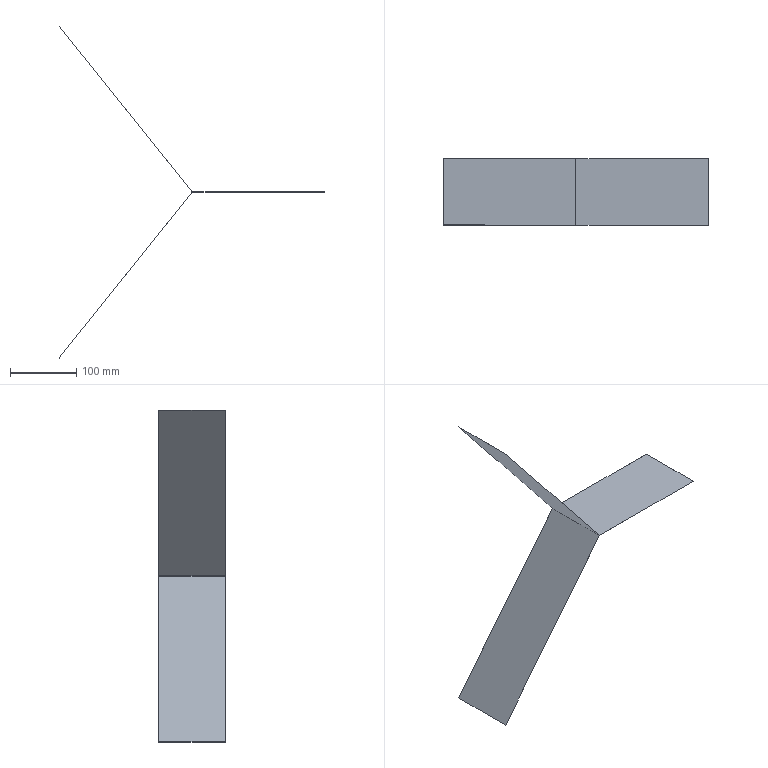Part | STEP file | A14-Product-1 | 1 solid | 11 faces | box 399.758 x 100 x 500.012 mm | volume 1680 mm3 | plane 11
STEP:
#1=CARTESIAN_POINT('',(0.,0.,0.));
#2=DIRECTION('',(0.,0.,1.));
#3=DIRECTION('',(1.,0.,0.));
#4=AXIS2_PLACEMENT_3D('',#1,#2,#3);
#5=CARTESIAN_POINT('',(199.755,-50.,0.01));
#6=VERTEX_POINT('',#5);
#7=CARTESIAN_POINT('',(399.75,-50.,0.01));
#8=VERTEX_POINT('',#7);
#9=CARTESIAN_POINT('',(199.75,-50.,0.01));
#10=DIRECTION('',(1.,0.,0.));
#11=VECTOR('',#10,1.);
#12=LINE('',#9,#11);
#13=CARTESIAN_POINT('',(0.,-50.,0.));
#14=DIRECTION('',(0.,-1.,0.));
#15=DIRECTION('',(-1.,0.,0.));
#16=AXIS2_PLACEMENT_3D('',#13,#14,#15);
#17=PLANE('',#16);
#18=CARTESIAN_POINT('',(-199.75,-0.01));
#19=DIRECTION('',(-1.,0.));
#20=VECTOR('',#19,1.);
#21=LINE('',#18,#20);
#22=(GEOMETRIC_REPRESENTATION_CONTEXT(2)PARAMETRIC_REPRESENTATION_CONTEXT()REPRESENTATION_CONTEXT('',''));
#23=DEFINITIONAL_REPRESENTATION('',(#21),#22);
#24=PCURVE('',#17,#23);
#25=CARTESIAN_POINT('',(199.75,50.,0.01));
#26=DIRECTION('',(0.,0.,-1.));
#27=DIRECTION('',(-1.,0.,0.));
#28=AXIS2_PLACEMENT_3D('',#25,#26,#27);
#29=PLANE('',#28);
#30=CARTESIAN_POINT('',(0.,-100.));
#31=DIRECTION('',(-1.,0.));
#32=VECTOR('',#31,1.);
#33=LINE('',#30,#32);
#34=(GEOMETRIC_REPRESENTATION_CONTEXT(2)PARAMETRIC_REPRESENTATION_CONTEXT()REPRESENTATION_CONTEXT('',''));
#35=DEFINITIONAL_REPRESENTATION('',(#33),#34);
#36=PCURVE('',#29,#35);
#37=SURFACE_CURVE('',#12,(#24,#36),.PCURVE_S1.);
#38=EDGE_CURVE('',#6,#8,#37,.T.);
#39=ORIENTED_EDGE('',*,*,#38,.F.);
#40=CARTESIAN_POINT('',(0.007812,-50.,250.006));
#41=VERTEX_POINT('',#40);
#42=CARTESIAN_POINT('',(199.758,-50.,0.006242));
#43=DIRECTION('',(-0.6242,0.,0.7812));
#44=VECTOR('',#43,1.);
#45=LINE('',#42,#44);
#46=CARTESIAN_POINT('',(-199.758,-0.006242));
#47=DIRECTION('',(0.6242,-0.7812));
#48=VECTOR('',#47,1.);
#49=LINE('',#46,#48);
#50=(GEOMETRIC_REPRESENTATION_CONTEXT(2)PARAMETRIC_REPRESENTATION_CONTEXT()REPRESENTATION_CONTEXT('',''));
#51=DEFINITIONAL_REPRESENTATION('',(#49),#50);
#52=PCURVE('',#17,#51);
#53=CARTESIAN_POINT('',(199.758,50.,0.006242));
#54=DIRECTION('',(0.7812,0.,0.6242));
#55=DIRECTION('',(0.6242,0.,-0.7812));
#56=AXIS2_PLACEMENT_3D('',#53,#54,#55);
#57=PLANE('',#56);
#58=CARTESIAN_POINT('',(0.,-100.));
#59=DIRECTION('',(-1.,0.));
#60=VECTOR('',#59,1.);
#61=LINE('',#58,#60);
#62=(GEOMETRIC_REPRESENTATION_CONTEXT(2)PARAMETRIC_REPRESENTATION_CONTEXT()REPRESENTATION_CONTEXT('',''));
#63=DEFINITIONAL_REPRESENTATION('',(#61),#62);
#64=PCURVE('',#57,#63);
#65=SURFACE_CURVE('',#45,(#52,#64),.PCURVE_S1.);
#66=EDGE_CURVE('',#6,#41,#65,.T.);
#67=ORIENTED_EDGE('',*,*,#66,.T.);
#68=CARTESIAN_POINT('',(-0.007813,-50.,249.994));
#69=VERTEX_POINT('',#68);
#70=CARTESIAN_POINT('',(0.007812,-50.,250.006));
#71=DIRECTION('',(-0.7812,0.,-0.6242));
#72=VECTOR('',#71,1.);
#73=LINE('',#70,#72);
#74=CARTESIAN_POINT('',(-0.007812,-250.006));
#75=DIRECTION('',(0.7812,0.6242));
#76=VECTOR('',#75,1.);
#77=LINE('',#74,#76);
#78=(GEOMETRIC_REPRESENTATION_CONTEXT(2)PARAMETRIC_REPRESENTATION_CONTEXT()REPRESENTATION_CONTEXT('',''));
#79=DEFINITIONAL_REPRESENTATION('',(#77),#78);
#80=PCURVE('',#17,#79);
#81=CARTESIAN_POINT('',(0.007812,50.,250.006));
#82=DIRECTION('',(-0.6242,0.,0.7812));
#83=DIRECTION('',(0.7812,0.,0.6242));
#84=AXIS2_PLACEMENT_3D('',#81,#82,#83);
#85=PLANE('',#84);
#86=CARTESIAN_POINT('',(0.,-100.));
#87=DIRECTION('',(-1.,0.));
#88=VECTOR('',#87,1.);
#89=LINE('',#86,#88);
#90=(GEOMETRIC_REPRESENTATION_CONTEXT(2)PARAMETRIC_REPRESENTATION_CONTEXT()REPRESENTATION_CONTEXT('',''));
#91=DEFINITIONAL_REPRESENTATION('',(#89),#90);
#92=PCURVE('',#85,#91);
#93=SURFACE_CURVE('',#73,(#80,#92),.PCURVE_S1.);
#94=EDGE_CURVE('',#41,#69,#93,.T.);
#95=ORIENTED_EDGE('',*,*,#94,.T.);
#96=CARTESIAN_POINT('',(199.737,-50.,0.));
#97=VERTEX_POINT('',#96);
#98=CARTESIAN_POINT('',(199.742,-50.,-0.006242));
#99=DIRECTION('',(-0.6242,0.,0.7812));
#100=VECTOR('',#99,1.);
#101=LINE('',#98,#100);
#102=CARTESIAN_POINT('',(-199.742,0.006242));
#103=DIRECTION('',(0.6242,-0.7812));
#104=VECTOR('',#103,1.);
#105=LINE('',#102,#104);
#106=(GEOMETRIC_REPRESENTATION_CONTEXT(2)PARAMETRIC_REPRESENTATION_CONTEXT()REPRESENTATION_CONTEXT('',''));
#107=DEFINITIONAL_REPRESENTATION('',(#105),#106);
#108=PCURVE('',#17,#107);
#109=CARTESIAN_POINT('',(199.742,50.,-0.006242));
#110=DIRECTION('',(0.7812,0.,0.6242));
#111=DIRECTION('',(0.6242,0.,-0.7812));
#112=AXIS2_PLACEMENT_3D('',#109,#110,#111);
#113=PLANE('',#112);
#114=CARTESIAN_POINT('',(0.,-100.));
#115=DIRECTION('',(-1.,0.));
#116=VECTOR('',#115,1.);
#117=LINE('',#114,#116);
#118=(GEOMETRIC_REPRESENTATION_CONTEXT(2)PARAMETRIC_REPRESENTATION_CONTEXT()REPRESENTATION_CONTEXT('',''));
#119=DEFINITIONAL_REPRESENTATION('',(#117),#118);
#120=PCURVE('',#113,#119);
#121=SURFACE_CURVE('',#101,(#108,#120),.PCURVE_S1.);
#122=EDGE_CURVE('',#97,#69,#121,.T.);
#123=ORIENTED_EDGE('',*,*,#122,.F.);
#124=CARTESIAN_POINT('',(-0.007812,-50.,-249.994));
#125=VERTEX_POINT('',#124);
#126=CARTESIAN_POINT('',(-0.007812,-50.,-249.994));
#127=DIRECTION('',(0.6242,0.,0.7812));
#128=VECTOR('',#127,1.);
#129=LINE('',#126,#128);
#130=CARTESIAN_POINT('',(0.007812,249.994));
#131=DIRECTION('',(-0.6242,-0.7812));
#132=VECTOR('',#131,1.);
#133=LINE('',#130,#132);
#134=(GEOMETRIC_REPRESENTATION_CONTEXT(2)PARAMETRIC_REPRESENTATION_CONTEXT()REPRESENTATION_CONTEXT('',''));
#135=DEFINITIONAL_REPRESENTATION('',(#133),#134);
#136=PCURVE('',#17,#135);
#137=CARTESIAN_POINT('',(-0.007812,50.,-249.994));
#138=DIRECTION('',(0.7812,0.,-0.6242));
#139=DIRECTION('',(-0.6242,0.,-0.7812));
#140=AXIS2_PLACEMENT_3D('',#137,#138,#139);
#141=PLANE('',#140);
#142=CARTESIAN_POINT('',(0.,-100.));
#143=DIRECTION('',(-1.,0.));
#144=VECTOR('',#143,1.);
#145=LINE('',#142,#144);
#146=(GEOMETRIC_REPRESENTATION_CONTEXT(2)PARAMETRIC_REPRESENTATION_CONTEXT()REPRESENTATION_CONTEXT('',''));
#147=DEFINITIONAL_REPRESENTATION('',(#145),#146);
#148=PCURVE('',#141,#147);
#149=SURFACE_CURVE('',#129,(#136,#148),.PCURVE_S1.);
#150=EDGE_CURVE('',#125,#97,#149,.T.);
#151=ORIENTED_EDGE('',*,*,#150,.F.);
#152=CARTESIAN_POINT('',(0.007813,-50.,-250.006));
#153=VERTEX_POINT('',#152);
#154=CARTESIAN_POINT('',(-0.007812,-50.,-249.994));
#155=DIRECTION('',(0.7812,0.,-0.6242));
#156=VECTOR('',#155,1.);
#157=LINE('',#154,#156);
#158=CARTESIAN_POINT('',(0.007812,249.994));
#159=DIRECTION('',(-0.7812,0.6242));
#160=VECTOR('',#159,1.);
#161=LINE('',#158,#160);
#162=(GEOMETRIC_REPRESENTATION_CONTEXT(2)PARAMETRIC_REPRESENTATION_CONTEXT()REPRESENTATION_CONTEXT('',''));
#163=DEFINITIONAL_REPRESENTATION('',(#161),#162);
#164=PCURVE('',#17,#163);
#165=CARTESIAN_POINT('',(-0.007812,50.,-249.994));
#166=DIRECTION('',(-0.6242,0.,-0.7812));
#167=DIRECTION('',(-0.7812,0.,0.6242));
#168=AXIS2_PLACEMENT_3D('',#165,#166,#167);
#169=PLANE('',#168);
#170=CARTESIAN_POINT('',(0.,-100.));
#171=DIRECTION('',(-1.,0.));
#172=VECTOR('',#171,1.);
#173=LINE('',#170,#172);
#174=(GEOMETRIC_REPRESENTATION_CONTEXT(2)PARAMETRIC_REPRESENTATION_CONTEXT()REPRESENTATION_CONTEXT('',''));
#175=DEFINITIONAL_REPRESENTATION('',(#173),#174);
#176=PCURVE('',#169,#175);
#177=SURFACE_CURVE('',#157,(#164,#176),.PCURVE_S1.);
#178=EDGE_CURVE('',#125,#153,#177,.T.);
#179=ORIENTED_EDGE('',*,*,#178,.T.);
#180=CARTESIAN_POINT('',(199.755,-50.,-0.01));
#181=VERTEX_POINT('',#180);
#182=CARTESIAN_POINT('',(0.007813,-50.,-250.006));
#183=DIRECTION('',(0.6242,0.,0.7812));
#184=VECTOR('',#183,1.);
#185=LINE('',#182,#184);
#186=CARTESIAN_POINT('',(-0.007813,250.006));
#187=DIRECTION('',(-0.6242,-0.7812));
#188=VECTOR('',#187,1.);
#189=LINE('',#186,#188);
#190=(GEOMETRIC_REPRESENTATION_CONTEXT(2)PARAMETRIC_REPRESENTATION_CONTEXT()REPRESENTATION_CONTEXT('',''));
#191=DEFINITIONAL_REPRESENTATION('',(#189),#190);
#192=PCURVE('',#17,#191);
#193=CARTESIAN_POINT('',(0.007813,50.,-250.006));
#194=DIRECTION('',(0.7812,0.,-0.6242));
#195=DIRECTION('',(-0.6242,0.,-0.7812));
#196=AXIS2_PLACEMENT_3D('',#193,#194,#195);
#197=PLANE('',#196);
#198=CARTESIAN_POINT('',(0.,-100.));
#199=DIRECTION('',(-1.,0.));
#200=VECTOR('',#199,1.);
#201=LINE('',#198,#200);
#202=(GEOMETRIC_REPRESENTATION_CONTEXT(2)PARAMETRIC_REPRESENTATION_CONTEXT()REPRESENTATION_CONTEXT('',''));
#203=DEFINITIONAL_REPRESENTATION('',(#201),#202);
#204=PCURVE('',#197,#203);
#205=SURFACE_CURVE('',#185,(#192,#204),.PCURVE_S1.);
#206=EDGE_CURVE('',#153,#181,#205,.T.);
#207=ORIENTED_EDGE('',*,*,#206,.T.);
#208=CARTESIAN_POINT('',(399.75,-50.,-0.01));
#209=VERTEX_POINT('',#208);
#210=CARTESIAN_POINT('',(199.75,-50.,-0.01));
#211=DIRECTION('',(1.,0.,0.));
#212=VECTOR('',#211,1.);
#213=LINE('',#210,#212);
#214=CARTESIAN_POINT('',(-199.75,0.01));
#215=DIRECTION('',(-1.,0.));
#216=VECTOR('',#215,1.);
#217=LINE('',#214,#216);
#218=(GEOMETRIC_REPRESENTATION_CONTEXT(2)PARAMETRIC_REPRESENTATION_CONTEXT()REPRESENTATION_CONTEXT('',''));
#219=DEFINITIONAL_REPRESENTATION('',(#217),#218);
#220=PCURVE('',#17,#219);
#221=CARTESIAN_POINT('',(199.75,50.,-0.01));
#222=DIRECTION('',(0.,0.,-1.));
#223=DIRECTION('',(-1.,0.,0.));
#224=AXIS2_PLACEMENT_3D('',#221,#222,#223);
#225=PLANE('',#224);
#226=CARTESIAN_POINT('',(0.,-100.));
#227=DIRECTION('',(-1.,0.));
#228=VECTOR('',#227,1.);
#229=LINE('',#226,#228);
#230=(GEOMETRIC_REPRESENTATION_CONTEXT(2)PARAMETRIC_REPRESENTATION_CONTEXT()REPRESENTATION_CONTEXT('',''));
#231=DEFINITIONAL_REPRESENTATION('',(#229),#230);
#232=PCURVE('',#225,#231);
#233=SURFACE_CURVE('',#213,(#220,#232),.PCURVE_S1.);
#234=EDGE_CURVE('',#181,#209,#233,.T.);
#235=ORIENTED_EDGE('',*,*,#234,.T.);
#236=CARTESIAN_POINT('',(399.75,-50.,-0.01));
#237=DIRECTION('',(0.,0.,1.));
#238=VECTOR('',#237,1.);
#239=LINE('',#236,#238);
#240=CARTESIAN_POINT('',(-399.75,0.01));
#241=DIRECTION('',(0.,-1.));
#242=VECTOR('',#241,1.);
#243=LINE('',#240,#242);
#244=(GEOMETRIC_REPRESENTATION_CONTEXT(2)PARAMETRIC_REPRESENTATION_CONTEXT()REPRESENTATION_CONTEXT('',''));
#245=DEFINITIONAL_REPRESENTATION('',(#243),#244);
#246=PCURVE('',#17,#245);
#247=CARTESIAN_POINT('',(399.75,50.,-0.01));
#248=DIRECTION('',(1.,0.,0.));
#249=DIRECTION('',(0.,0.,-1.));
#250=AXIS2_PLACEMENT_3D('',#247,#248,#249);
#251=PLANE('',#250);
#252=CARTESIAN_POINT('',(0.,-100.));
#253=DIRECTION('',(-1.,0.));
#254=VECTOR('',#253,1.);
#255=LINE('',#252,#254);
#256=(GEOMETRIC_REPRESENTATION_CONTEXT(2)PARAMETRIC_REPRESENTATION_CONTEXT()REPRESENTATION_CONTEXT('',''));
#257=DEFINITIONAL_REPRESENTATION('',(#255),#256);
#258=PCURVE('',#251,#257);
#259=SURFACE_CURVE('',#239,(#246,#258),.PCURVE_S1.);
#260=EDGE_CURVE('',#209,#8,#259,.T.);
#261=ORIENTED_EDGE('',*,*,#260,.T.);
#262=EDGE_LOOP('',(#39,#67,#95,#123,#151,#179,#207,#235,#261));
#263=FACE_BOUND('',#262,.T.);
#264=ADVANCED_FACE('',(#263),#17,.T.);
#265=CARTESIAN_POINT('',(199.755,50.,-0.01));
#266=VERTEX_POINT('',#265);
#267=CARTESIAN_POINT('',(199.755,50.,-0.01));
#268=DIRECTION('',(0.,1.,0.));
#269=VECTOR('',#268,1.);
#270=LINE('',#267,#269);
#271=CARTESIAN_POINT('',(-319.995,0.));
#272=DIRECTION('',(0.,1.));
#273=VECTOR('',#272,1.);
#274=LINE('',#271,#273);
#275=(GEOMETRIC_REPRESENTATION_CONTEXT(2)PARAMETRIC_REPRESENTATION_CONTEXT()REPRESENTATION_CONTEXT('',''));
#276=DEFINITIONAL_REPRESENTATION('',(#274),#275);
#277=PCURVE('',#197,#276);
#278=CARTESIAN_POINT('',(-0.00481,0.));
#279=DIRECTION('',(0.,1.));
#280=VECTOR('',#279,1.);
#281=LINE('',#278,#280);
#282=(GEOMETRIC_REPRESENTATION_CONTEXT(2)PARAMETRIC_REPRESENTATION_CONTEXT()REPRESENTATION_CONTEXT('',''));
#283=DEFINITIONAL_REPRESENTATION('',(#281),#282);
#284=PCURVE('',#225,#283);
#285=SURFACE_CURVE('',#270,(#277,#284),.PCURVE_S1.);
#286=EDGE_CURVE('',#181,#266,#285,.T.);
#287=ORIENTED_EDGE('',*,*,#286,.F.);
#288=ORIENTED_EDGE('',*,*,#206,.F.);
#289=CARTESIAN_POINT('',(0.007813,50.,-250.006));
#290=VERTEX_POINT('',#289);
#291=CARTESIAN_POINT('',(0.007813,50.,-250.006));
#292=DIRECTION('',(0.,-1.,0.));
#293=VECTOR('',#292,1.);
#294=LINE('',#291,#293);
#295=CARTESIAN_POINT('',(0.,0.));
#296=DIRECTION('',(0.,-1.));
#297=VECTOR('',#296,1.);
#298=LINE('',#295,#297);
#299=(GEOMETRIC_REPRESENTATION_CONTEXT(2)PARAMETRIC_REPRESENTATION_CONTEXT()REPRESENTATION_CONTEXT('',''));
#300=DEFINITIONAL_REPRESENTATION('',(#298),#299);
#301=PCURVE('',#197,#300);
#302=CARTESIAN_POINT('',(-0.02,0.));
#303=DIRECTION('',(0.,-1.));
#304=VECTOR('',#303,1.);
#305=LINE('',#302,#304);
#306=(GEOMETRIC_REPRESENTATION_CONTEXT(2)PARAMETRIC_REPRESENTATION_CONTEXT()REPRESENTATION_CONTEXT('',''));
#307=DEFINITIONAL_REPRESENTATION('',(#305),#306);
#308=PCURVE('',#169,#307);
#309=SURFACE_CURVE('',#294,(#301,#308),.PCURVE_S1.);
#310=EDGE_CURVE('',#290,#153,#309,.T.);
#311=ORIENTED_EDGE('',*,*,#310,.F.);
#312=CARTESIAN_POINT('',(0.007813,50.,-250.006));
#313=DIRECTION('',(0.6242,0.,0.7812));
#314=VECTOR('',#313,1.);
#315=LINE('',#312,#314);
#316=CARTESIAN_POINT('',(0.,0.));
#317=DIRECTION('',(-1.,0.));
#318=VECTOR('',#317,1.);
#319=LINE('',#316,#318);
#320=(GEOMETRIC_REPRESENTATION_CONTEXT(2)PARAMETRIC_REPRESENTATION_CONTEXT()REPRESENTATION_CONTEXT('',''));
#321=DEFINITIONAL_REPRESENTATION('',(#319),#320);
#322=PCURVE('',#197,#321);
#323=CARTESIAN_POINT('',(0.,50.,0.));
#324=DIRECTION('',(0.,-1.,0.));
#325=DIRECTION('',(-1.,0.,0.));
#326=AXIS2_PLACEMENT_3D('',#323,#324,#325);
#327=PLANE('',#326);
#328=CARTESIAN_POINT('',(-0.007813,250.006));
#329=DIRECTION('',(-0.6242,-0.7812));
#330=VECTOR('',#329,1.);
#331=LINE('',#328,#330);
#332=(GEOMETRIC_REPRESENTATION_CONTEXT(2)PARAMETRIC_REPRESENTATION_CONTEXT()REPRESENTATION_CONTEXT('',''));
#333=DEFINITIONAL_REPRESENTATION('',(#331),#332);
#334=PCURVE('',#327,#333);
#335=SURFACE_CURVE('',#315,(#322,#334),.PCURVE_S1.);
#336=EDGE_CURVE('',#290,#266,#335,.T.);
#337=ORIENTED_EDGE('',*,*,#336,.T.);
#338=EDGE_LOOP('',(#287,#288,#311,#337));
#339=FACE_BOUND('',#338,.T.);
#340=ADVANCED_FACE('',(#339),#197,.T.);
#341=ORIENTED_EDGE('',*,*,#178,.F.);
#342=CARTESIAN_POINT('',(-0.007812,50.,-249.994));
#343=VERTEX_POINT('',#342);
#344=CARTESIAN_POINT('',(-0.007812,50.,-249.994));
#345=DIRECTION('',(0.,-1.,0.));
#346=VECTOR('',#345,1.);
#347=LINE('',#344,#346);
#348=CARTESIAN_POINT('',(0.,0.));
#349=DIRECTION('',(0.,-1.));
#350=VECTOR('',#349,1.);
#351=LINE('',#348,#350);
#352=(GEOMETRIC_REPRESENTATION_CONTEXT(2)PARAMETRIC_REPRESENTATION_CONTEXT()REPRESENTATION_CONTEXT('',''));
#353=DEFINITIONAL_REPRESENTATION('',(#351),#352);
#354=PCURVE('',#169,#353);
#355=CARTESIAN_POINT('',(0.,0.));
#356=DIRECTION('',(0.,-1.));
#357=VECTOR('',#356,1.);
#358=LINE('',#355,#357);
#359=(GEOMETRIC_REPRESENTATION_CONTEXT(2)PARAMETRIC_REPRESENTATION_CONTEXT()REPRESENTATION_CONTEXT('',''));
#360=DEFINITIONAL_REPRESENTATION('',(#358),#359);
#361=PCURVE('',#141,#360);
#362=SURFACE_CURVE('',#347,(#354,#361),.PCURVE_S1.);
#363=EDGE_CURVE('',#343,#125,#362,.T.);
#364=ORIENTED_EDGE('',*,*,#363,.F.);
#365=CARTESIAN_POINT('',(-0.007812,50.,-249.994));
#366=DIRECTION('',(0.7812,0.,-0.6242));
#367=VECTOR('',#366,1.);
#368=LINE('',#365,#367);
#369=CARTESIAN_POINT('',(0.,0.));
#370=DIRECTION('',(-1.,0.));
#371=VECTOR('',#370,1.);
#372=LINE('',#369,#371);
#373=(GEOMETRIC_REPRESENTATION_CONTEXT(2)PARAMETRIC_REPRESENTATION_CONTEXT()REPRESENTATION_CONTEXT('',''));
#374=DEFINITIONAL_REPRESENTATION('',(#372),#373);
#375=PCURVE('',#169,#374);
#376=CARTESIAN_POINT('',(0.007812,249.994));
#377=DIRECTION('',(-0.7812,0.6242));
#378=VECTOR('',#377,1.);
#379=LINE('',#376,#378);
#380=(GEOMETRIC_REPRESENTATION_CONTEXT(2)PARAMETRIC_REPRESENTATION_CONTEXT()REPRESENTATION_CONTEXT('',''));
#381=DEFINITIONAL_REPRESENTATION('',(#379),#380);
#382=PCURVE('',#327,#381);
#383=SURFACE_CURVE('',#368,(#375,#382),.PCURVE_S1.);
#384=EDGE_CURVE('',#343,#290,#383,.T.);
#385=ORIENTED_EDGE('',*,*,#384,.T.);
#386=ORIENTED_EDGE('',*,*,#310,.T.);
#387=EDGE_LOOP('',(#341,#364,#385,#386));
#388=FACE_BOUND('',#387,.T.);
#389=ADVANCED_FACE('',(#388),#169,.T.);
#390=CARTESIAN_POINT('',(199.737,50.,0.));
#391=VERTEX_POINT('',#390);
#392=CARTESIAN_POINT('',(199.737,50.,0.));
#393=DIRECTION('',(0.,-1.,0.));
#394=VECTOR('',#393,1.);
#395=LINE('',#392,#394);
#396=CARTESIAN_POINT('',(-319.992,0.));
#397=DIRECTION('',(0.,-1.));
#398=VECTOR('',#397,1.);
#399=LINE('',#396,#398);
#400=(GEOMETRIC_REPRESENTATION_CONTEXT(2)PARAMETRIC_REPRESENTATION_CONTEXT()REPRESENTATION_CONTEXT('',''));
#401=DEFINITIONAL_REPRESENTATION('',(#399),#400);
#402=PCURVE('',#141,#401);
#403=CARTESIAN_POINT('',(-0.00799,0.));
#404=DIRECTION('',(0.,-1.));
#405=VECTOR('',#404,1.);
#406=LINE('',#403,#405);
#407=(GEOMETRIC_REPRESENTATION_CONTEXT(2)PARAMETRIC_REPRESENTATION_CONTEXT()REPRESENTATION_CONTEXT('',''));
#408=DEFINITIONAL_REPRESENTATION('',(#406),#407);
#409=PCURVE('',#113,#408);
#410=SURFACE_CURVE('',#395,(#402,#409),.PCURVE_S1.);
#411=EDGE_CURVE('',#391,#97,#410,.T.);
#412=ORIENTED_EDGE('',*,*,#411,.F.);
#413=CARTESIAN_POINT('',(-0.007812,50.,-249.994));
#414=DIRECTION('',(0.6242,0.,0.7812));
#415=VECTOR('',#414,1.);
#416=LINE('',#413,#415);
#417=CARTESIAN_POINT('',(0.,0.));
#418=DIRECTION('',(-1.,0.));
#419=VECTOR('',#418,1.);
#420=LINE('',#417,#419);
#421=(GEOMETRIC_REPRESENTATION_CONTEXT(2)PARAMETRIC_REPRESENTATION_CONTEXT()REPRESENTATION_CONTEXT('',''));
#422=DEFINITIONAL_REPRESENTATION('',(#420),#421);
#423=PCURVE('',#141,#422);
#424=CARTESIAN_POINT('',(0.007812,249.994));
#425=DIRECTION('',(-0.6242,-0.7812));
#426=VECTOR('',#425,1.);
#427=LINE('',#424,#426);
#428=(GEOMETRIC_REPRESENTATION_CONTEXT(2)PARAMETRIC_REPRESENTATION_CONTEXT()REPRESENTATION_CONTEXT('',''));
#429=DEFINITIONAL_REPRESENTATION('',(#427),#428);
#430=PCURVE('',#327,#429);
#431=SURFACE_CURVE('',#416,(#423,#430),.PCURVE_S1.);
#432=EDGE_CURVE('',#343,#391,#431,.T.);
#433=ORIENTED_EDGE('',*,*,#432,.F.);
#434=ORIENTED_EDGE('',*,*,#363,.T.);
#435=ORIENTED_EDGE('',*,*,#150,.T.);
#436=EDGE_LOOP('',(#412,#433,#434,#435));
#437=FACE_BOUND('',#436,.T.);
#438=ADVANCED_FACE('',(#437),#141,.F.);
#439=CARTESIAN_POINT('',(199.755,50.,0.01));
#440=VERTEX_POINT('',#439);
#441=CARTESIAN_POINT('',(0.007812,50.,250.006));
#442=VERTEX_POINT('',#441);
#443=CARTESIAN_POINT('',(199.758,50.,0.006242));
#444=DIRECTION('',(-0.6242,0.,0.7812));
#445=VECTOR('',#444,1.);
#446=LINE('',#443,#445);
#447=CARTESIAN_POINT('',(-199.758,-0.006242));
#448=DIRECTION('',(0.6242,-0.7812));
#449=VECTOR('',#448,1.);
#450=LINE('',#447,#449);
#451=(GEOMETRIC_REPRESENTATION_CONTEXT(2)PARAMETRIC_REPRESENTATION_CONTEXT()REPRESENTATION_CONTEXT('',''));
#452=DEFINITIONAL_REPRESENTATION('',(#450),#451);
#453=PCURVE('',#327,#452);
#454=CARTESIAN_POINT('',(0.,0.));
#455=DIRECTION('',(-1.,0.));
#456=VECTOR('',#455,1.);
#457=LINE('',#454,#456);
#458=(GEOMETRIC_REPRESENTATION_CONTEXT(2)PARAMETRIC_REPRESENTATION_CONTEXT()REPRESENTATION_CONTEXT('',''));
#459=DEFINITIONAL_REPRESENTATION('',(#457),#458);
#460=PCURVE('',#57,#459);
#461=SURFACE_CURVE('',#446,(#453,#460),.PCURVE_S1.);
#462=EDGE_CURVE('',#440,#442,#461,.T.);
#463=ORIENTED_EDGE('',*,*,#462,.F.);
#464=CARTESIAN_POINT('',(399.75,50.,0.01));
#465=VERTEX_POINT('',#464);
#466=CARTESIAN_POINT('',(199.75,50.,0.01));
#467=DIRECTION('',(1.,0.,0.));
#468=VECTOR('',#467,1.);
#469=LINE('',#466,#468);
#470=CARTESIAN_POINT('',(-199.75,-0.01));
#471=DIRECTION('',(-1.,0.));
#472=VECTOR('',#471,1.);
#473=LINE('',#470,#472);
#474=(GEOMETRIC_REPRESENTATION_CONTEXT(2)PARAMETRIC_REPRESENTATION_CONTEXT()REPRESENTATION_CONTEXT('',''));
#475=DEFINITIONAL_REPRESENTATION('',(#473),#474);
#476=PCURVE('',#327,#475);
#477=CARTESIAN_POINT('',(0.,0.));
#478=DIRECTION('',(-1.,0.));
#479=VECTOR('',#478,1.);
#480=LINE('',#477,#479);
#481=(GEOMETRIC_REPRESENTATION_CONTEXT(2)PARAMETRIC_REPRESENTATION_CONTEXT()REPRESENTATION_CONTEXT('',''));
#482=DEFINITIONAL_REPRESENTATION('',(#480),#481);
#483=PCURVE('',#29,#482);
#484=SURFACE_CURVE('',#469,(#476,#483),.PCURVE_S1.);
#485=EDGE_CURVE('',#440,#465,#484,.T.);
#486=ORIENTED_EDGE('',*,*,#485,.T.);
#487=CARTESIAN_POINT('',(399.75,50.,-0.01));
#488=VERTEX_POINT('',#487);
#489=CARTESIAN_POINT('',(399.75,50.,-0.01));
#490=DIRECTION('',(0.,0.,1.));
#491=VECTOR('',#490,1.);
#492=LINE('',#489,#491);
#493=CARTESIAN_POINT('',(-399.75,0.01));
#494=DIRECTION('',(0.,-1.));
#495=VECTOR('',#494,1.);
#496=LINE('',#493,#495);
#497=(GEOMETRIC_REPRESENTATION_CONTEXT(2)PARAMETRIC_REPRESENTATION_CONTEXT()REPRESENTATION_CONTEXT('',''));
#498=DEFINITIONAL_REPRESENTATION('',(#496),#497);
#499=PCURVE('',#327,#498);
#500=CARTESIAN_POINT('',(0.,0.));
#501=DIRECTION('',(-1.,0.));
#502=VECTOR('',#501,1.);
#503=LINE('',#500,#502);
#504=(GEOMETRIC_REPRESENTATION_CONTEXT(2)PARAMETRIC_REPRESENTATION_CONTEXT()REPRESENTATION_CONTEXT('',''));
#505=DEFINITIONAL_REPRESENTATION('',(#503),#504);
#506=PCURVE('',#251,#505);
#507=SURFACE_CURVE('',#492,(#499,#506),.PCURVE_S1.);
#508=EDGE_CURVE('',#488,#465,#507,.T.);
#509=ORIENTED_EDGE('',*,*,#508,.F.);
#510=CARTESIAN_POINT('',(199.75,50.,-0.01));
#511=DIRECTION('',(1.,0.,0.));
#512=VECTOR('',#511,1.);
#513=LINE('',#510,#512);
#514=CARTESIAN_POINT('',(-199.75,0.01));
#515=DIRECTION('',(-1.,0.));
#516=VECTOR('',#515,1.);
#517=LINE('',#514,#516);
#518=(GEOMETRIC_REPRESENTATION_CONTEXT(2)PARAMETRIC_REPRESENTATION_CONTEXT()REPRESENTATION_CONTEXT('',''));
#519=DEFINITIONAL_REPRESENTATION('',(#517),#518);
#520=PCURVE('',#327,#519);
#521=CARTESIAN_POINT('',(0.,0.));
#522=DIRECTION('',(-1.,0.));
#523=VECTOR('',#522,1.);
#524=LINE('',#521,#523);
#525=(GEOMETRIC_REPRESENTATION_CONTEXT(2)PARAMETRIC_REPRESENTATION_CONTEXT()REPRESENTATION_CONTEXT('',''));
#526=DEFINITIONAL_REPRESENTATION('',(#524),#525);
#527=PCURVE('',#225,#526);
#528=SURFACE_CURVE('',#513,(#520,#527),.PCURVE_S1.);
#529=EDGE_CURVE('',#266,#488,#528,.T.);
#530=ORIENTED_EDGE('',*,*,#529,.F.);
#531=ORIENTED_EDGE('',*,*,#336,.F.);
#532=ORIENTED_EDGE('',*,*,#384,.F.);
#533=ORIENTED_EDGE('',*,*,#432,.T.);
#534=CARTESIAN_POINT('',(-0.007813,50.,249.994));
#535=VERTEX_POINT('',#534);
#536=CARTESIAN_POINT('',(199.742,50.,-0.006242));
#537=DIRECTION('',(-0.6242,0.,0.7812));
#538=VECTOR('',#537,1.);
#539=LINE('',#536,#538);
#540=CARTESIAN_POINT('',(-199.742,0.006242));
#541=DIRECTION('',(0.6242,-0.7812));
#542=VECTOR('',#541,1.);
#543=LINE('',#540,#542);
#544=(GEOMETRIC_REPRESENTATION_CONTEXT(2)PARAMETRIC_REPRESENTATION_CONTEXT()REPRESENTATION_CONTEXT('',''));
#545=DEFINITIONAL_REPRESENTATION('',(#543),#544);
#546=PCURVE('',#327,#545);
#547=CARTESIAN_POINT('',(0.,0.));
#548=DIRECTION('',(-1.,0.));
#549=VECTOR('',#548,1.);
#550=LINE('',#547,#549);
#551=(GEOMETRIC_REPRESENTATION_CONTEXT(2)PARAMETRIC_REPRESENTATION_CONTEXT()REPRESENTATION_CONTEXT('',''));
#552=DEFINITIONAL_REPRESENTATION('',(#550),#551);
#553=PCURVE('',#113,#552);
#554=SURFACE_CURVE('',#539,(#546,#553),.PCURVE_S1.);
#555=EDGE_CURVE('',#391,#535,#554,.T.);
#556=ORIENTED_EDGE('',*,*,#555,.T.);
#557=CARTESIAN_POINT('',(0.007812,50.,250.006));
#558=DIRECTION('',(-0.7812,0.,-0.6242));
#559=VECTOR('',#558,1.);
#560=LINE('',#557,#559);
#561=CARTESIAN_POINT('',(-0.007812,-250.006));
#562=DIRECTION('',(0.7812,0.6242));
#563=VECTOR('',#562,1.);
#564=LINE('',#561,#563);
#565=(GEOMETRIC_REPRESENTATION_CONTEXT(2)PARAMETRIC_REPRESENTATION_CONTEXT()REPRESENTATION_CONTEXT('',''));
#566=DEFINITIONAL_REPRESENTATION('',(#564),#565);
#567=PCURVE('',#327,#566);
#568=CARTESIAN_POINT('',(0.,0.));
#569=DIRECTION('',(-1.,0.));
#570=VECTOR('',#569,1.);
#571=LINE('',#568,#570);
#572=(GEOMETRIC_REPRESENTATION_CONTEXT(2)PARAMETRIC_REPRESENTATION_CONTEXT()REPRESENTATION_CONTEXT('',''));
#573=DEFINITIONAL_REPRESENTATION('',(#571),#572);
#574=PCURVE('',#85,#573);
#575=SURFACE_CURVE('',#560,(#567,#574),.PCURVE_S1.);
#576=EDGE_CURVE('',#442,#535,#575,.T.);
#577=ORIENTED_EDGE('',*,*,#576,.F.);
#578=EDGE_LOOP('',(#463,#486,#509,#530,#531,#532,#533,#556,#577));
#579=FACE_BOUND('',#578,.T.);
#580=ADVANCED_FACE('',(#579),#327,.F.);
#581=ORIENTED_EDGE('',*,*,#94,.F.);
#582=CARTESIAN_POINT('',(0.007812,50.,250.006));
#583=DIRECTION('',(0.,-1.,0.));
#584=VECTOR('',#583,1.);
#585=LINE('',#582,#584);
#586=CARTESIAN_POINT('',(0.,0.));
#587=DIRECTION('',(0.,-1.));
#588=VECTOR('',#587,1.);
#589=LINE('',#586,#588);
#590=(GEOMETRIC_REPRESENTATION_CONTEXT(2)PARAMETRIC_REPRESENTATION_CONTEXT()REPRESENTATION_CONTEXT('',''));
#591=DEFINITIONAL_REPRESENTATION('',(#589),#590);
#592=PCURVE('',#85,#591);
#593=CARTESIAN_POINT('',(-320.,0.));
#594=DIRECTION('',(0.,-1.));
#595=VECTOR('',#594,1.);
#596=LINE('',#593,#595);
#597=(GEOMETRIC_REPRESENTATION_CONTEXT(2)PARAMETRIC_REPRESENTATION_CONTEXT()REPRESENTATION_CONTEXT('',''));
#598=DEFINITIONAL_REPRESENTATION('',(#596),#597);
#599=PCURVE('',#57,#598);
#600=SURFACE_CURVE('',#585,(#592,#599),.PCURVE_S1.);
#601=EDGE_CURVE('',#442,#41,#600,.T.);
#602=ORIENTED_EDGE('',*,*,#601,.F.);
#603=ORIENTED_EDGE('',*,*,#576,.T.);
#604=CARTESIAN_POINT('',(-0.007813,50.,249.994));
#605=DIRECTION('',(0.,-1.,0.));
#606=VECTOR('',#605,1.);
#607=LINE('',#604,#606);
#608=CARTESIAN_POINT('',(-0.02,0.));
#609=DIRECTION('',(0.,-1.));
#610=VECTOR('',#609,1.);
#611=LINE('',#608,#610);
#612=(GEOMETRIC_REPRESENTATION_CONTEXT(2)PARAMETRIC_REPRESENTATION_CONTEXT()REPRESENTATION_CONTEXT('',''));
#613=DEFINITIONAL_REPRESENTATION('',(#611),#612);
#614=PCURVE('',#85,#613);
#615=CARTESIAN_POINT('',(-320.,0.));
#616=DIRECTION('',(0.,-1.));
#617=VECTOR('',#616,1.);
#618=LINE('',#615,#617);
#619=(GEOMETRIC_REPRESENTATION_CONTEXT(2)PARAMETRIC_REPRESENTATION_CONTEXT()REPRESENTATION_CONTEXT('',''));
#620=DEFINITIONAL_REPRESENTATION('',(#618),#619);
#621=PCURVE('',#113,#620);
#622=SURFACE_CURVE('',#607,(#614,#621),.PCURVE_S1.);
#623=EDGE_CURVE('',#535,#69,#622,.T.);
#624=ORIENTED_EDGE('',*,*,#623,.T.);
#625=EDGE_LOOP('',(#581,#602,#603,#624));
#626=FACE_BOUND('',#625,.T.);
#627=ADVANCED_FACE('',(#626),#85,.T.);
#628=CARTESIAN_POINT('',(199.755,50.,0.01));
#629=DIRECTION('',(0.,-1.,0.));
#630=VECTOR('',#629,1.);
#631=LINE('',#628,#630);
#632=CARTESIAN_POINT('',(-0.00481,0.));
#633=DIRECTION('',(0.,-1.));
#634=VECTOR('',#633,1.);
#635=LINE('',#632,#634);
#636=(GEOMETRIC_REPRESENTATION_CONTEXT(2)PARAMETRIC_REPRESENTATION_CONTEXT()REPRESENTATION_CONTEXT('',''));
#637=DEFINITIONAL_REPRESENTATION('',(#635),#636);
#638=PCURVE('',#57,#637);
#639=CARTESIAN_POINT('',(-0.00481,0.));
#640=DIRECTION('',(0.,-1.));
#641=VECTOR('',#640,1.);
#642=LINE('',#639,#641);
#643=(GEOMETRIC_REPRESENTATION_CONTEXT(2)PARAMETRIC_REPRESENTATION_CONTEXT()REPRESENTATION_CONTEXT('',''));
#644=DEFINITIONAL_REPRESENTATION('',(#642),#643);
#645=PCURVE('',#29,#644);
#646=SURFACE_CURVE('',#631,(#638,#645),.PCURVE_S1.);
#647=EDGE_CURVE('',#440,#6,#646,.T.);
#648=ORIENTED_EDGE('',*,*,#647,.F.);
#649=ORIENTED_EDGE('',*,*,#462,.T.);
#650=ORIENTED_EDGE('',*,*,#601,.T.);
#651=ORIENTED_EDGE('',*,*,#66,.F.);
#652=EDGE_LOOP('',(#648,#649,#650,#651));
#653=FACE_BOUND('',#652,.T.);
#654=ADVANCED_FACE('',(#653),#57,.T.);
#655=ORIENTED_EDGE('',*,*,#555,.F.);
#656=ORIENTED_EDGE('',*,*,#411,.T.);
#657=ORIENTED_EDGE('',*,*,#122,.T.);
#658=ORIENTED_EDGE('',*,*,#623,.F.);
#659=EDGE_LOOP('',(#655,#656,#657,#658));
#660=FACE_BOUND('',#659,.T.);
#661=ADVANCED_FACE('',(#660),#113,.F.);
#662=ORIENTED_EDGE('',*,*,#485,.F.);
#663=ORIENTED_EDGE('',*,*,#647,.T.);
#664=ORIENTED_EDGE('',*,*,#38,.T.);
#665=CARTESIAN_POINT('',(399.75,50.,0.01));
#666=DIRECTION('',(0.,-1.,0.));
#667=VECTOR('',#666,1.);
#668=LINE('',#665,#667);
#669=CARTESIAN_POINT('',(-200.,0.));
#670=DIRECTION('',(0.,-1.));
#671=VECTOR('',#670,1.);
#672=LINE('',#669,#671);
#673=(GEOMETRIC_REPRESENTATION_CONTEXT(2)PARAMETRIC_REPRESENTATION_CONTEXT()REPRESENTATION_CONTEXT('',''));
#674=DEFINITIONAL_REPRESENTATION('',(#672),#673);
#675=PCURVE('',#29,#674);
#676=CARTESIAN_POINT('',(-0.02,0.));
#677=DIRECTION('',(0.,-1.));
#678=VECTOR('',#677,1.);
#679=LINE('',#676,#678);
#680=(GEOMETRIC_REPRESENTATION_CONTEXT(2)PARAMETRIC_REPRESENTATION_CONTEXT()REPRESENTATION_CONTEXT('',''));
#681=DEFINITIONAL_REPRESENTATION('',(#679),#680);
#682=PCURVE('',#251,#681);
#683=SURFACE_CURVE('',#668,(#675,#682),.PCURVE_S1.);
#684=EDGE_CURVE('',#465,#8,#683,.T.);
#685=ORIENTED_EDGE('',*,*,#684,.F.);
#686=EDGE_LOOP('',(#662,#663,#664,#685));
#687=FACE_BOUND('',#686,.T.);
#688=ADVANCED_FACE('',(#687),#29,.F.);
#689=ORIENTED_EDGE('',*,*,#260,.F.);
#690=CARTESIAN_POINT('',(399.75,50.,-0.01));
#691=DIRECTION('',(0.,-1.,0.));
#692=VECTOR('',#691,1.);
#693=LINE('',#690,#692);
#694=CARTESIAN_POINT('',(0.,0.));
#695=DIRECTION('',(0.,-1.));
#696=VECTOR('',#695,1.);
#697=LINE('',#694,#696);
#698=(GEOMETRIC_REPRESENTATION_CONTEXT(2)PARAMETRIC_REPRESENTATION_CONTEXT()REPRESENTATION_CONTEXT('',''));
#699=DEFINITIONAL_REPRESENTATION('',(#697),#698);
#700=PCURVE('',#251,#699);
#701=CARTESIAN_POINT('',(-200.,0.));
#702=DIRECTION('',(0.,-1.));
#703=VECTOR('',#702,1.);
#704=LINE('',#701,#703);
#705=(GEOMETRIC_REPRESENTATION_CONTEXT(2)PARAMETRIC_REPRESENTATION_CONTEXT()REPRESENTATION_CONTEXT('',''));
#706=DEFINITIONAL_REPRESENTATION('',(#704),#705);
#707=PCURVE('',#225,#706);
#708=SURFACE_CURVE('',#693,(#700,#707),.PCURVE_S1.);
#709=EDGE_CURVE('',#488,#209,#708,.T.);
#710=ORIENTED_EDGE('',*,*,#709,.F.);
#711=ORIENTED_EDGE('',*,*,#508,.T.);
#712=ORIENTED_EDGE('',*,*,#684,.T.);
#713=EDGE_LOOP('',(#689,#710,#711,#712));
#714=FACE_BOUND('',#713,.T.);
#715=ADVANCED_FACE('',(#714),#251,.T.);
#716=ORIENTED_EDGE('',*,*,#234,.F.);
#717=ORIENTED_EDGE('',*,*,#286,.T.);
#718=ORIENTED_EDGE('',*,*,#529,.T.);
#719=ORIENTED_EDGE('',*,*,#709,.T.);
#720=EDGE_LOOP('',(#716,#717,#718,#719));
#721=FACE_BOUND('',#720,.T.);
#722=ADVANCED_FACE('',(#721),#225,.T.);
#723=CLOSED_SHELL('',(#264,#340,#389,#438,#580,#627,#654,#661,#688,#715,#722));
#724=MANIFOLD_SOLID_BREP('',#723);
#725=(LENGTH_UNIT()NAMED_UNIT(*)SI_UNIT(.MILLI.,.METRE.));
#726=UNCERTAINTY_MEASURE_WITH_UNIT(LENGTH_MEASURE(0.0000001),#725,'','');
#727=(NAMED_UNIT(*)PLANE_ANGLE_UNIT()SI_UNIT($,.RADIAN.));
#728=(NAMED_UNIT(*)SI_UNIT($,.STERADIAN.)SOLID_ANGLE_UNIT());
#729=(GEOMETRIC_REPRESENTATION_CONTEXT(3)GLOBAL_UNCERTAINTY_ASSIGNED_CONTEXT((#726))GLOBAL_UNIT_ASSIGNED_CONTEXT((#725,#727,#728))REPRESENTATION_CONTEXT('',''));
#730=ADVANCED_BREP_SHAPE_REPRESENTATION('',(#4,#724),#729);